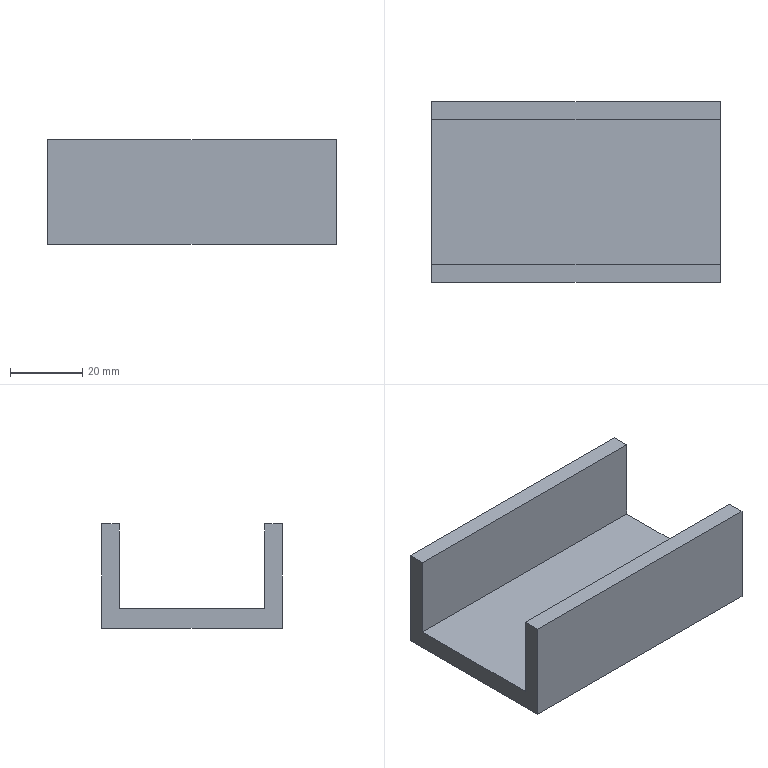Part | SolidWorks | features Extrusion 1, ICE 1 | 1 solid | 10 faces | box 80 x 50 x 28.83 mm | volume 39671 mm3 | plane 10
STEP:
#1=CARTESIAN_POINT('',(80.,0.,28.83));
#2=VERTEX_POINT('',#1);
#3=CARTESIAN_POINT('',(80.,4.855,28.83));
#4=VERTEX_POINT('',#3);
#5=CARTESIAN_POINT('',(80.,0.,28.83));
#6=DIRECTION('',(0.,1.,0.));
#7=VECTOR('',#6,1000.);
#8=LINE('',#5,#7);
#9=EDGE_CURVE('',#2,#4,#8,.T.);
#10=ORIENTED_EDGE('',*,*,#9,.T.);
#11=CARTESIAN_POINT('',(0.,4.855,28.83));
#12=VERTEX_POINT('',#11);
#13=CARTESIAN_POINT('',(0.,4.855,28.83));
#14=DIRECTION('',(1.,0.,0.));
#15=VECTOR('',#14,1000.);
#16=LINE('',#13,#15);
#17=EDGE_CURVE('',#12,#4,#16,.T.);
#18=ORIENTED_EDGE('',*,*,#17,.F.);
#19=CARTESIAN_POINT('',(0.,0.,28.83));
#20=VERTEX_POINT('',#19);
#21=CARTESIAN_POINT('',(0.,0.,28.83));
#22=DIRECTION('',(0.,-1.,0.));
#23=VECTOR('',#22,1000.);
#24=LINE('',#21,#23);
#25=EDGE_CURVE('',#12,#20,#24,.T.);
#26=ORIENTED_EDGE('',*,*,#25,.T.);
#27=CARTESIAN_POINT('',(0.,0.,28.83));
#28=DIRECTION('',(1.,0.,0.));
#29=VECTOR('',#28,1000.);
#30=LINE('',#27,#29);
#31=EDGE_CURVE('',#20,#2,#30,.T.);
#32=ORIENTED_EDGE('',*,*,#31,.T.);
#33=EDGE_LOOP('',(#10,#18,#26,#32));
#34=FACE_OUTER_BOUND('',#33,.T.);
#35=CARTESIAN_POINT('',(0.,0.,28.83));
#36=DIRECTION('',(0.,0.,-1.));
#37=DIRECTION('',(-1.,0.,0.));
#38=AXIS2_PLACEMENT_3D('',#35,#36,#37);
#39=PLANE('',#38);
#40=ADVANCED_FACE('',(#34),#39,.F.);
#41=ORIENTED_EDGE('',*,*,#25,.F.);
#42=CARTESIAN_POINT('',(0.,4.855,5.362));
#43=VERTEX_POINT('',#42);
#44=CARTESIAN_POINT('',(0.,4.855,5.362));
#45=DIRECTION('',(0.,0.,-1.));
#46=VECTOR('',#45,1000.);
#47=LINE('',#44,#46);
#48=EDGE_CURVE('',#12,#43,#47,.T.);
#49=ORIENTED_EDGE('',*,*,#48,.T.);
#50=CARTESIAN_POINT('',(0.,45.149,5.362));
#51=VERTEX_POINT('',#50);
#52=CARTESIAN_POINT('',(0.,45.149,5.362));
#53=DIRECTION('',(0.,1.,0.));
#54=VECTOR('',#53,1000.);
#55=LINE('',#52,#54);
#56=EDGE_CURVE('',#43,#51,#55,.T.);
#57=ORIENTED_EDGE('',*,*,#56,.T.);
#58=CARTESIAN_POINT('',(0.,45.149,28.83));
#59=VERTEX_POINT('',#58);
#60=CARTESIAN_POINT('',(0.,45.149,5.362));
#61=DIRECTION('',(0.,0.,1.));
#62=VECTOR('',#61,1000.);
#63=LINE('',#60,#62);
#64=EDGE_CURVE('',#51,#59,#63,.T.);
#65=ORIENTED_EDGE('',*,*,#64,.T.);
#66=CARTESIAN_POINT('',(0.,50.,28.83));
#67=VERTEX_POINT('',#66);
#68=CARTESIAN_POINT('',(0.,0.,28.83));
#69=DIRECTION('',(0.,-1.,0.));
#70=VECTOR('',#69,1000.);
#71=LINE('',#68,#70);
#72=EDGE_CURVE('',#67,#59,#71,.T.);
#73=ORIENTED_EDGE('',*,*,#72,.F.);
#74=CARTESIAN_POINT('',(0.,50.,0.));
#75=VERTEX_POINT('',#74);
#76=CARTESIAN_POINT('',(0.,50.,28.83));
#77=DIRECTION('',(0.,0.,-1.));
#78=VECTOR('',#77,1000.);
#79=LINE('',#76,#78);
#80=EDGE_CURVE('',#67,#75,#79,.T.);
#81=ORIENTED_EDGE('',*,*,#80,.T.);
#82=CARTESIAN_POINT('',(0.,0.,0.));
#83=VERTEX_POINT('',#82);
#84=CARTESIAN_POINT('',(0.,0.,0.));
#85=DIRECTION('',(0.,-1.,0.));
#86=VECTOR('',#85,1000.);
#87=LINE('',#84,#86);
#88=EDGE_CURVE('',#75,#83,#87,.T.);
#89=ORIENTED_EDGE('',*,*,#88,.T.);
#90=CARTESIAN_POINT('',(0.,0.,28.83));
#91=DIRECTION('',(0.,0.,-1.));
#92=VECTOR('',#91,1000.);
#93=LINE('',#90,#92);
#94=EDGE_CURVE('',#20,#83,#93,.T.);
#95=ORIENTED_EDGE('',*,*,#94,.F.);
#96=EDGE_LOOP('',(#41,#49,#57,#65,#73,#81,#89,#95));
#97=FACE_OUTER_BOUND('',#96,.T.);
#98=CARTESIAN_POINT('',(0.,0.,28.83));
#99=DIRECTION('',(1.,0.,0.));
#100=DIRECTION('',(0.,0.,-1.));
#101=AXIS2_PLACEMENT_3D('',#98,#99,#100);
#102=PLANE('',#101);
#103=ADVANCED_FACE('',(#97),#102,.F.);
#104=CARTESIAN_POINT('',(80.,0.,0.));
#105=VERTEX_POINT('',#104);
#106=CARTESIAN_POINT('',(0.,0.,0.));
#107=DIRECTION('',(1.,0.,0.));
#108=VECTOR('',#107,1000.);
#109=LINE('',#106,#108);
#110=EDGE_CURVE('',#83,#105,#109,.T.);
#111=ORIENTED_EDGE('',*,*,#110,.T.);
#112=CARTESIAN_POINT('',(80.,0.,28.83));
#113=DIRECTION('',(0.,0.,-1.));
#114=VECTOR('',#113,1000.);
#115=LINE('',#112,#114);
#116=EDGE_CURVE('',#2,#105,#115,.T.);
#117=ORIENTED_EDGE('',*,*,#116,.F.);
#118=ORIENTED_EDGE('',*,*,#31,.F.);
#119=ORIENTED_EDGE('',*,*,#94,.T.);
#120=EDGE_LOOP('',(#111,#117,#118,#119));
#121=FACE_OUTER_BOUND('',#120,.T.);
#122=CARTESIAN_POINT('',(0.,0.,28.83));
#123=DIRECTION('',(0.,1.,0.));
#124=DIRECTION('',(0.,0.,1.));
#125=AXIS2_PLACEMENT_3D('',#122,#123,#124);
#126=PLANE('',#125);
#127=ADVANCED_FACE('',(#121),#126,.F.);
#128=CARTESIAN_POINT('',(80.,4.855,5.362));
#129=VERTEX_POINT('',#128);
#130=CARTESIAN_POINT('',(80.,45.149,5.362));
#131=VERTEX_POINT('',#130);
#132=CARTESIAN_POINT('',(80.,45.149,5.362));
#133=DIRECTION('',(0.,1.,0.));
#134=VECTOR('',#133,1000.);
#135=LINE('',#132,#134);
#136=EDGE_CURVE('',#129,#131,#135,.T.);
#137=ORIENTED_EDGE('',*,*,#136,.F.);
#138=CARTESIAN_POINT('',(80.,4.855,5.362));
#139=DIRECTION('',(0.,0.,-1.));
#140=VECTOR('',#139,1000.);
#141=LINE('',#138,#140);
#142=EDGE_CURVE('',#4,#129,#141,.T.);
#143=ORIENTED_EDGE('',*,*,#142,.F.);
#144=ORIENTED_EDGE('',*,*,#9,.F.);
#145=ORIENTED_EDGE('',*,*,#116,.T.);
#146=CARTESIAN_POINT('',(80.,50.,0.));
#147=VERTEX_POINT('',#146);
#148=CARTESIAN_POINT('',(80.,0.,0.));
#149=DIRECTION('',(0.,1.,0.));
#150=VECTOR('',#149,1000.);
#151=LINE('',#148,#150);
#152=EDGE_CURVE('',#105,#147,#151,.T.);
#153=ORIENTED_EDGE('',*,*,#152,.T.);
#154=CARTESIAN_POINT('',(80.,50.,28.83));
#155=VERTEX_POINT('',#154);
#156=CARTESIAN_POINT('',(80.,50.,28.83));
#157=DIRECTION('',(0.,0.,-1.));
#158=VECTOR('',#157,1000.);
#159=LINE('',#156,#158);
#160=EDGE_CURVE('',#155,#147,#159,.T.);
#161=ORIENTED_EDGE('',*,*,#160,.F.);
#162=CARTESIAN_POINT('',(80.,45.149,28.83));
#163=VERTEX_POINT('',#162);
#164=CARTESIAN_POINT('',(80.,0.,28.83));
#165=DIRECTION('',(0.,1.,0.));
#166=VECTOR('',#165,1000.);
#167=LINE('',#164,#166);
#168=EDGE_CURVE('',#163,#155,#167,.T.);
#169=ORIENTED_EDGE('',*,*,#168,.F.);
#170=CARTESIAN_POINT('',(80.,45.149,5.362));
#171=DIRECTION('',(0.,0.,1.));
#172=VECTOR('',#171,1000.);
#173=LINE('',#170,#172);
#174=EDGE_CURVE('',#131,#163,#173,.T.);
#175=ORIENTED_EDGE('',*,*,#174,.F.);
#176=EDGE_LOOP('',(#137,#143,#144,#145,#153,#161,#169,#175));
#177=FACE_OUTER_BOUND('',#176,.T.);
#178=CARTESIAN_POINT('',(80.,0.,28.83));
#179=DIRECTION('',(-1.,0.,0.));
#180=DIRECTION('',(0.,0.,1.));
#181=AXIS2_PLACEMENT_3D('',#178,#179,#180);
#182=PLANE('',#181);
#183=ADVANCED_FACE('',(#177),#182,.F.);
#184=CARTESIAN_POINT('',(0.,50.,0.));
#185=DIRECTION('',(-1.,0.,0.));
#186=VECTOR('',#185,1000.);
#187=LINE('',#184,#186);
#188=EDGE_CURVE('',#147,#75,#187,.T.);
#189=ORIENTED_EDGE('',*,*,#188,.T.);
#190=ORIENTED_EDGE('',*,*,#80,.F.);
#191=CARTESIAN_POINT('',(0.,50.,28.83));
#192=DIRECTION('',(-1.,0.,0.));
#193=VECTOR('',#192,1000.);
#194=LINE('',#191,#193);
#195=EDGE_CURVE('',#155,#67,#194,.T.);
#196=ORIENTED_EDGE('',*,*,#195,.F.);
#197=ORIENTED_EDGE('',*,*,#160,.T.);
#198=EDGE_LOOP('',(#189,#190,#196,#197));
#199=FACE_OUTER_BOUND('',#198,.T.);
#200=CARTESIAN_POINT('',(0.,50.,28.83));
#201=DIRECTION('',(0.,-1.,0.));
#202=DIRECTION('',(0.,0.,-1.));
#203=AXIS2_PLACEMENT_3D('',#200,#201,#202);
#204=PLANE('',#203);
#205=ADVANCED_FACE('',(#199),#204,.F.);
#206=ORIENTED_EDGE('',*,*,#72,.T.);
#207=CARTESIAN_POINT('',(0.,45.149,28.83));
#208=DIRECTION('',(1.,0.,0.));
#209=VECTOR('',#208,1000.);
#210=LINE('',#207,#209);
#211=EDGE_CURVE('',#59,#163,#210,.T.);
#212=ORIENTED_EDGE('',*,*,#211,.T.);
#213=ORIENTED_EDGE('',*,*,#168,.T.);
#214=ORIENTED_EDGE('',*,*,#195,.T.);
#215=EDGE_LOOP('',(#206,#212,#213,#214));
#216=FACE_OUTER_BOUND('',#215,.T.);
#217=CARTESIAN_POINT('',(0.,0.,28.83));
#218=DIRECTION('',(0.,0.,-1.));
#219=DIRECTION('',(-1.,0.,0.));
#220=AXIS2_PLACEMENT_3D('',#217,#218,#219);
#221=PLANE('',#220);
#222=ADVANCED_FACE('',(#216),#221,.F.);
#223=ORIENTED_EDGE('',*,*,#88,.F.);
#224=ORIENTED_EDGE('',*,*,#188,.F.);
#225=ORIENTED_EDGE('',*,*,#152,.F.);
#226=ORIENTED_EDGE('',*,*,#110,.F.);
#227=EDGE_LOOP('',(#223,#224,#225,#226));
#228=FACE_OUTER_BOUND('',#227,.T.);
#229=CARTESIAN_POINT('',(0.,0.,0.));
#230=DIRECTION('',(0.,0.,-1.));
#231=DIRECTION('',(-1.,0.,0.));
#232=AXIS2_PLACEMENT_3D('',#229,#230,#231);
#233=PLANE('',#232);
#234=ADVANCED_FACE('',(#228),#233,.T.);
#235=ORIENTED_EDGE('',*,*,#136,.T.);
#236=CARTESIAN_POINT('',(0.,45.149,5.362));
#237=DIRECTION('',(1.,0.,0.));
#238=VECTOR('',#237,1000.);
#239=LINE('',#236,#238);
#240=EDGE_CURVE('',#51,#131,#239,.T.);
#241=ORIENTED_EDGE('',*,*,#240,.F.);
#242=ORIENTED_EDGE('',*,*,#56,.F.);
#243=CARTESIAN_POINT('',(0.,4.855,5.362));
#244=DIRECTION('',(1.,0.,0.));
#245=VECTOR('',#244,1000.);
#246=LINE('',#243,#245);
#247=EDGE_CURVE('',#43,#129,#246,.T.);
#248=ORIENTED_EDGE('',*,*,#247,.T.);
#249=EDGE_LOOP('',(#235,#241,#242,#248));
#250=FACE_OUTER_BOUND('',#249,.T.);
#251=CARTESIAN_POINT('',(0.,45.149,5.362));
#252=DIRECTION('',(0.,0.,-1.));
#253=DIRECTION('',(-1.,0.,0.));
#254=AXIS2_PLACEMENT_3D('',#251,#252,#253);
#255=PLANE('',#254);
#256=ADVANCED_FACE('',(#250),#255,.F.);
#257=ORIENTED_EDGE('',*,*,#142,.T.);
#258=ORIENTED_EDGE('',*,*,#247,.F.);
#259=ORIENTED_EDGE('',*,*,#48,.F.);
#260=ORIENTED_EDGE('',*,*,#17,.T.);
#261=EDGE_LOOP('',(#257,#258,#259,#260));
#262=FACE_OUTER_BOUND('',#261,.T.);
#263=CARTESIAN_POINT('',(0.,4.855,5.362));
#264=DIRECTION('',(0.,-1.,0.));
#265=DIRECTION('',(0.,0.,-1.));
#266=AXIS2_PLACEMENT_3D('',#263,#264,#265);
#267=PLANE('',#266);
#268=ADVANCED_FACE('',(#262),#267,.F.);
#269=ORIENTED_EDGE('',*,*,#174,.T.);
#270=ORIENTED_EDGE('',*,*,#211,.F.);
#271=ORIENTED_EDGE('',*,*,#64,.F.);
#272=ORIENTED_EDGE('',*,*,#240,.T.);
#273=EDGE_LOOP('',(#269,#270,#271,#272));
#274=FACE_OUTER_BOUND('',#273,.T.);
#275=CARTESIAN_POINT('',(0.,45.149,5.362));
#276=DIRECTION('',(0.,1.,0.));
#277=DIRECTION('',(0.,0.,1.));
#278=AXIS2_PLACEMENT_3D('',#275,#276,#277);
#279=PLANE('',#278);
#280=ADVANCED_FACE('',(#274),#279,.F.);
#281=CLOSED_SHELL('',(#40,#103,#127,#183,#205,#222,#234,#256,#268,#280));
#282=MANIFOLD_SOLID_BREP('',#281);
#283=CARTESIAN_POINT('',(0.,0.,0.));
#284=DIRECTION('',(0.,0.,1.));
#285=DIRECTION('',(1.,0.,0.));
#286=AXIS2_PLACEMENT_3D('',#283,#284,#285);
#287=(LENGTH_UNIT()NAMED_UNIT(*)SI_UNIT(.MILLI.,.METRE.));
#288=UNCERTAINTY_MEASURE_WITH_UNIT(LENGTH_MEASURE(0.00001),#287,'','');
#289=(NAMED_UNIT(*)PLANE_ANGLE_UNIT()SI_UNIT($,.RADIAN.));
#290=(NAMED_UNIT(*)SI_UNIT($,.STERADIAN.)SOLID_ANGLE_UNIT());
#291=(GEOMETRIC_REPRESENTATION_CONTEXT(3)GLOBAL_UNCERTAINTY_ASSIGNED_CONTEXT((#288))GLOBAL_UNIT_ASSIGNED_CONTEXT((#287,#289,#290))REPRESENTATION_CONTEXT('',''));
#292=ADVANCED_BREP_SHAPE_REPRESENTATION('',(#282,#286),#291);